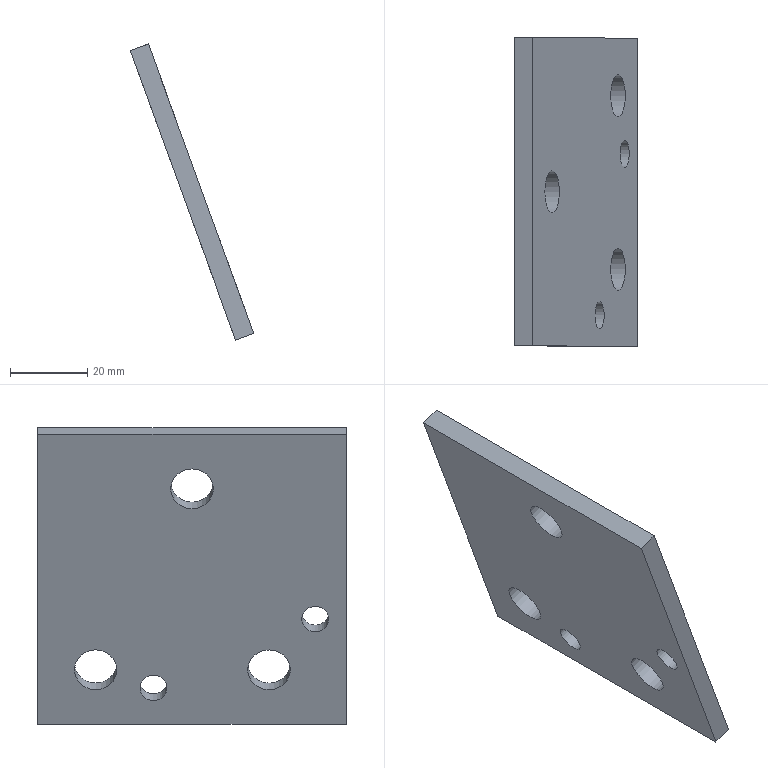Part | NX | features solid 2 | 1 solid | 11 faces | box 32.064 x 80.011 x 76.896 mm | volume 30190 mm3 | plane 6 | cylinder 5 | commonest cylinder face diameters 11 x3 7 x2
STEP:
#1=CARTESIAN_POINT('',(730.878,-346.999,86.488));
#2=VERTEX_POINT('',#1);
#3=CARTESIAN_POINT('',(758.239,-346.988,11.313));
#4=VERTEX_POINT('',#3);
#5=CARTESIAN_POINT('',(759.949,-346.987,6.614));
#6=DIRECTION('',(0.342,0.0001374,-0.9397));
#7=VECTOR('',#6,1000.);
#8=LINE('',#5,#7);
#9=EDGE_CURVE('',#2,#4,#8,.T.);
#10=ORIENTED_EDGE('',*,*,#9,.F.);
#11=CARTESIAN_POINT('',(726.179,-346.999,84.778));
#12=VERTEX_POINT('',#11);
#13=CARTESIAN_POINT('',(726.179,-346.999,84.778));
#14=DIRECTION('',(0.9397,-0.000001517,0.342));
#15=VECTOR('',#14,1000.);
#16=LINE('',#13,#15);
#17=EDGE_CURVE('',#12,#2,#16,.T.);
#18=ORIENTED_EDGE('',*,*,#17,.F.);
#19=CARTESIAN_POINT('',(753.541,-346.988,9.603));
#20=VERTEX_POINT('',#19);
#21=CARTESIAN_POINT('',(755.251,-346.987,4.904));
#22=DIRECTION('',(0.342,0.0001374,-0.9397));
#23=VECTOR('',#22,1000.);
#24=LINE('',#21,#23);
#25=EDGE_CURVE('',#12,#20,#24,.T.);
#26=ORIENTED_EDGE('',*,*,#25,.T.);
#27=CARTESIAN_POINT('',(753.541,-346.988,9.603));
#28=DIRECTION('',(0.9397,-0.000001517,0.342));
#29=VECTOR('',#28,1000.);
#30=LINE('',#27,#29);
#31=EDGE_CURVE('',#20,#4,#30,.T.);
#32=ORIENTED_EDGE('',*,*,#31,.T.);
#33=EDGE_LOOP('',(#10,#18,#26,#32));
#34=FACE_BOUND('',#33,.T.);
#35=CARTESIAN_POINT('',(755.251,-346.987,4.904));
#36=DIRECTION('',(-0.00004556,1.,0.0001296));
#37=DIRECTION('',(0.000000501,-0.0001296,1.));
#38=AXIS2_PLACEMENT_3D('',#35,#36,#37);
#39=PLANE('',#38);
#40=ADVANCED_FACE('',(#34),#39,.F.);
#41=CARTESIAN_POINT('',(730.874,-266.999,86.498));
#42=VERTEX_POINT('',#41);
#43=CARTESIAN_POINT('',(730.873,-236.999,86.502));
#44=DIRECTION('',(0.00004556,-1.,-0.0001296));
#45=VECTOR('',#44,1000.);
#46=LINE('',#43,#45);
#47=EDGE_CURVE('',#42,#2,#46,.T.);
#48=ORIENTED_EDGE('',*,*,#47,.F.);
#49=CARTESIAN_POINT('',(726.176,-266.999,84.788));
#50=VERTEX_POINT('',#49);
#51=CARTESIAN_POINT('',(726.176,-266.999,84.788));
#52=DIRECTION('',(0.9397,-0.000001517,0.342));
#53=VECTOR('',#52,1000.);
#54=LINE('',#51,#53);
#55=EDGE_CURVE('',#50,#42,#54,.T.);
#56=ORIENTED_EDGE('',*,*,#55,.F.);
#57=CARTESIAN_POINT('',(726.174,-236.999,84.792));
#58=DIRECTION('',(0.00004556,-1.,-0.0001296));
#59=VECTOR('',#58,1000.);
#60=LINE('',#57,#59);
#61=EDGE_CURVE('',#50,#12,#60,.T.);
#62=ORIENTED_EDGE('',*,*,#61,.T.);
#63=ORIENTED_EDGE('',*,*,#17,.T.);
#64=EDGE_LOOP('',(#48,#56,#62,#63));
#65=FACE_BOUND('',#64,.T.);
#66=CARTESIAN_POINT('',(726.174,-236.999,84.792));
#67=DIRECTION('',(0.342,0.0001374,-0.9397));
#68=DIRECTION('',(0.9397,-0.000001517,0.342));
#69=AXIS2_PLACEMENT_3D('',#66,#67,#68);
#70=PLANE('',#69);
#71=ADVANCED_FACE('',(#65),#70,.F.);
#72=CARTESIAN_POINT('',(758.236,-266.988,11.323));
#73=VERTEX_POINT('',#72);
#74=CARTESIAN_POINT('',(759.946,-266.987,6.625));
#75=DIRECTION('',(-0.342,-0.0001374,0.9397));
#76=VECTOR('',#75,1000.);
#77=LINE('',#74,#76);
#78=EDGE_CURVE('',#73,#42,#77,.T.);
#79=ORIENTED_EDGE('',*,*,#78,.F.);
#80=CARTESIAN_POINT('',(753.537,-266.988,9.613));
#81=VERTEX_POINT('',#80);
#82=CARTESIAN_POINT('',(753.537,-266.988,9.613));
#83=DIRECTION('',(0.9397,-0.000001517,0.342));
#84=VECTOR('',#83,1000.);
#85=LINE('',#82,#84);
#86=EDGE_CURVE('',#81,#73,#85,.T.);
#87=ORIENTED_EDGE('',*,*,#86,.F.);
#88=CARTESIAN_POINT('',(755.247,-266.987,4.914));
#89=DIRECTION('',(-0.342,-0.0001374,0.9397));
#90=VECTOR('',#89,1000.);
#91=LINE('',#88,#90);
#92=EDGE_CURVE('',#81,#50,#91,.T.);
#93=ORIENTED_EDGE('',*,*,#92,.T.);
#94=ORIENTED_EDGE('',*,*,#55,.T.);
#95=EDGE_LOOP('',(#79,#87,#93,#94));
#96=FACE_BOUND('',#95,.T.);
#97=CARTESIAN_POINT('',(755.247,-266.987,4.914));
#98=DIRECTION('',(0.00004556,-1.,-0.0001296));
#99=DIRECTION('',(-0.000000501,0.0001296,-1.));
#100=AXIS2_PLACEMENT_3D('',#97,#98,#99);
#101=PLANE('',#100);
#102=ADVANCED_FACE('',(#96),#101,.F.);
#103=CARTESIAN_POINT('',(758.234,-236.988,11.327));
#104=DIRECTION('',(-0.00004556,1.,0.0001296));
#105=VECTOR('',#104,1000.);
#106=LINE('',#103,#105);
#107=EDGE_CURVE('',#4,#73,#106,.T.);
#108=ORIENTED_EDGE('',*,*,#107,.F.);
#109=ORIENTED_EDGE('',*,*,#31,.F.);
#110=CARTESIAN_POINT('',(753.536,-236.988,9.617));
#111=DIRECTION('',(-0.00004556,1.,0.0001296));
#112=VECTOR('',#111,1000.);
#113=LINE('',#110,#112);
#114=EDGE_CURVE('',#20,#81,#113,.T.);
#115=ORIENTED_EDGE('',*,*,#114,.T.);
#116=ORIENTED_EDGE('',*,*,#86,.T.);
#117=EDGE_LOOP('',(#108,#109,#115,#116));
#118=FACE_BOUND('',#117,.T.);
#119=CARTESIAN_POINT('',(753.536,-236.988,9.617));
#120=DIRECTION('',(-0.342,-0.0001374,0.9397));
#121=DIRECTION('',(-0.9397,0.000001517,-0.342));
#122=AXIS2_PLACEMENT_3D('',#119,#120,#121);
#123=PLANE('',#122);
#124=ADVANCED_FACE('',(#118),#123,.F.);
#125=CARTESIAN_POINT('',(729.427,-306.997,75.856));
#126=VERTEX_POINT('',#125);
#127=CARTESIAN_POINT('',(731.308,-306.997,70.688));
#128=DIRECTION('',(-0.9397,0.000001517,-0.342));
#129=DIRECTION('',(-0.342,0.,0.9397));
#130=AXIS2_PLACEMENT_3D('',#127,#128,#129);
#131=CIRCLE('',#130,5.5);
#132=EDGE_CURVE('',#126,#126,#131,.T.);
#133=ORIENTED_EDGE('',*,*,#132,.F.);
#134=EDGE_LOOP('',(#133));
#135=FACE_BOUND('',#134,.T.);
#136=CARTESIAN_POINT('',(742.425,-338.992,40.144));
#137=VERTEX_POINT('',#136);
#138=CARTESIAN_POINT('',(743.622,-338.992,36.855));
#139=DIRECTION('',(-0.9397,0.000001517,-0.342));
#140=DIRECTION('',(-0.342,0.,0.9397));
#141=AXIS2_PLACEMENT_3D('',#138,#139,#140);
#142=CIRCLE('',#141,3.5);
#143=EDGE_CURVE('',#137,#137,#142,.T.);
#144=ORIENTED_EDGE('',*,*,#143,.F.);
#145=EDGE_LOOP('',(#144));
#146=FACE_BOUND('',#145,.T.);
#147=CARTESIAN_POINT('',(746.528,-326.99,28.869));
#148=VERTEX_POINT('',#147);
#149=CARTESIAN_POINT('',(748.41,-326.99,23.701));
#150=DIRECTION('',(-0.9397,0.000001517,-0.342));
#151=DIRECTION('',(-0.342,0.00000071,0.9397));
#152=AXIS2_PLACEMENT_3D('',#149,#150,#151);
#153=CIRCLE('',#152,5.5);
#154=EDGE_CURVE('',#148,#148,#153,.T.);
#155=ORIENTED_EDGE('',*,*,#154,.F.);
#156=EDGE_LOOP('',(#155));
#157=FACE_BOUND('',#156,.T.);
#158=CARTESIAN_POINT('',(748.921,-296.989,22.295));
#159=VERTEX_POINT('',#158);
#160=CARTESIAN_POINT('',(750.118,-296.989,19.006));
#161=DIRECTION('',(-0.9397,0.000001517,-0.342));
#162=DIRECTION('',(-0.342,0.,0.9397));
#163=AXIS2_PLACEMENT_3D('',#160,#161,#162);
#164=CIRCLE('',#163,3.5);
#165=EDGE_CURVE('',#159,#159,#164,.T.);
#166=ORIENTED_EDGE('',*,*,#165,.F.);
#167=EDGE_LOOP('',(#166));
#168=FACE_BOUND('',#167,.T.);
#169=CARTESIAN_POINT('',(746.526,-281.99,28.875));
#170=VERTEX_POINT('',#169);
#171=CARTESIAN_POINT('',(748.407,-281.99,23.706));
#172=DIRECTION('',(-0.9397,0.000001517,-0.342));
#173=DIRECTION('',(-0.342,0.00000071,0.9397));
#174=AXIS2_PLACEMENT_3D('',#171,#172,#173);
#175=CIRCLE('',#174,5.5);
#176=EDGE_CURVE('',#170,#170,#175,.T.);
#177=ORIENTED_EDGE('',*,*,#176,.F.);
#178=EDGE_LOOP('',(#177));
#179=FACE_BOUND('',#178,.T.);
#180=ORIENTED_EDGE('',*,*,#25,.F.);
#181=ORIENTED_EDGE('',*,*,#61,.F.);
#182=ORIENTED_EDGE('',*,*,#92,.F.);
#183=ORIENTED_EDGE('',*,*,#114,.F.);
#184=EDGE_LOOP('',(#180,#181,#182,#183));
#185=FACE_BOUND('',#184,.T.);
#186=CARTESIAN_POINT('',(755.246,-236.987,4.918));
#187=DIRECTION('',(0.9397,-0.000001517,0.342));
#188=DIRECTION('',(-0.342,-0.0001374,0.9397));
#189=AXIS2_PLACEMENT_3D('',#186,#187,#188);
#190=PLANE('',#189);
#191=ADVANCED_FACE('',(#135,#146,#157,#168,#179,#185),#190,.F.);
#192=CARTESIAN_POINT('',(734.125,-306.997,77.566));
#193=VERTEX_POINT('',#192);
#194=CARTESIAN_POINT('',(736.006,-306.997,72.398));
#195=DIRECTION('',(-0.9397,0.000001517,-0.342));
#196=DIRECTION('',(-0.342,0.,0.9397));
#197=AXIS2_PLACEMENT_3D('',#194,#195,#196);
#198=CIRCLE('',#197,5.5);
#199=EDGE_CURVE('',#193,#193,#198,.T.);
#200=ORIENTED_EDGE('',*,*,#199,.T.);
#201=EDGE_LOOP('',(#200));
#202=FACE_BOUND('',#201,.T.);
#203=CARTESIAN_POINT('',(747.123,-338.992,41.854));
#204=VERTEX_POINT('',#203);
#205=CARTESIAN_POINT('',(748.32,-338.992,38.565));
#206=DIRECTION('',(-0.9397,0.000001517,-0.342));
#207=DIRECTION('',(-0.342,0.,0.9397));
#208=AXIS2_PLACEMENT_3D('',#205,#206,#207);
#209=CIRCLE('',#208,3.5);
#210=EDGE_CURVE('',#204,#204,#209,.T.);
#211=ORIENTED_EDGE('',*,*,#210,.T.);
#212=EDGE_LOOP('',(#211));
#213=FACE_BOUND('',#212,.T.);
#214=CARTESIAN_POINT('',(751.227,-326.99,30.579));
#215=VERTEX_POINT('',#214);
#216=CARTESIAN_POINT('',(753.108,-326.99,25.411));
#217=DIRECTION('',(-0.9397,0.000001517,-0.342));
#218=DIRECTION('',(-0.342,0.00000071,0.9397));
#219=AXIS2_PLACEMENT_3D('',#216,#217,#218);
#220=CIRCLE('',#219,5.5);
#221=EDGE_CURVE('',#215,#215,#220,.T.);
#222=ORIENTED_EDGE('',*,*,#221,.T.);
#223=EDGE_LOOP('',(#222));
#224=FACE_BOUND('',#223,.T.);
#225=CARTESIAN_POINT('',(753.62,-296.989,24.005));
#226=VERTEX_POINT('',#225);
#227=CARTESIAN_POINT('',(754.817,-296.989,20.716));
#228=DIRECTION('',(-0.9397,0.000001517,-0.342));
#229=DIRECTION('',(-0.342,0.,0.9397));
#230=AXIS2_PLACEMENT_3D('',#227,#228,#229);
#231=CIRCLE('',#230,3.5);
#232=EDGE_CURVE('',#226,#226,#231,.T.);
#233=ORIENTED_EDGE('',*,*,#232,.T.);
#234=EDGE_LOOP('',(#233));
#235=FACE_BOUND('',#234,.T.);
#236=CARTESIAN_POINT('',(751.225,-281.99,30.585));
#237=VERTEX_POINT('',#236);
#238=CARTESIAN_POINT('',(753.106,-281.99,25.416));
#239=DIRECTION('',(-0.9397,0.000001517,-0.342));
#240=DIRECTION('',(-0.342,0.00000071,0.9397));
#241=AXIS2_PLACEMENT_3D('',#238,#239,#240);
#242=CIRCLE('',#241,5.5);
#243=EDGE_CURVE('',#237,#237,#242,.T.);
#244=ORIENTED_EDGE('',*,*,#243,.T.);
#245=EDGE_LOOP('',(#244));
#246=FACE_BOUND('',#245,.T.);
#247=ORIENTED_EDGE('',*,*,#9,.T.);
#248=ORIENTED_EDGE('',*,*,#107,.T.);
#249=ORIENTED_EDGE('',*,*,#78,.T.);
#250=ORIENTED_EDGE('',*,*,#47,.T.);
#251=EDGE_LOOP('',(#247,#248,#249,#250));
#252=FACE_BOUND('',#251,.T.);
#253=CARTESIAN_POINT('',(759.944,-236.987,6.628));
#254=DIRECTION('',(0.9397,-0.000001517,0.342));
#255=DIRECTION('',(-0.342,-0.0001374,0.9397));
#256=AXIS2_PLACEMENT_3D('',#253,#254,#255);
#257=PLANE('',#256);
#258=ADVANCED_FACE('',(#202,#213,#224,#235,#246,#252),#257,.T.);
#259=ORIENTED_EDGE('',*,*,#243,.F.);
#260=EDGE_LOOP('',(#259));
#261=FACE_BOUND('',#260,.T.);
#262=ORIENTED_EDGE('',*,*,#176,.T.);
#263=EDGE_LOOP('',(#262));
#264=FACE_BOUND('',#263,.T.);
#265=CARTESIAN_POINT('',(743.709,-281.99,21.996));
#266=DIRECTION('',(0.9397,-0.000001517,0.342));
#267=DIRECTION('',(-0.342,0.00000071,0.9397));
#268=AXIS2_PLACEMENT_3D('',#265,#266,#267);
#269=CYLINDRICAL_SURFACE('',#268,5.5);
#270=ADVANCED_FACE('',(#261,#264),#269,.F.);
#271=ORIENTED_EDGE('',*,*,#232,.F.);
#272=EDGE_LOOP('',(#271));
#273=FACE_BOUND('',#272,.T.);
#274=ORIENTED_EDGE('',*,*,#165,.T.);
#275=EDGE_LOOP('',(#274));
#276=FACE_BOUND('',#275,.T.);
#277=CARTESIAN_POINT('',(745.42,-296.989,17.296));
#278=DIRECTION('',(0.9397,-0.000001517,0.342));
#279=DIRECTION('',(-0.342,0.00000071,0.9397));
#280=AXIS2_PLACEMENT_3D('',#277,#278,#279);
#281=CYLINDRICAL_SURFACE('',#280,3.5);
#282=ADVANCED_FACE('',(#273,#276),#281,.F.);
#283=ORIENTED_EDGE('',*,*,#221,.F.);
#284=EDGE_LOOP('',(#283));
#285=FACE_BOUND('',#284,.T.);
#286=ORIENTED_EDGE('',*,*,#154,.T.);
#287=EDGE_LOOP('',(#286));
#288=FACE_BOUND('',#287,.T.);
#289=CARTESIAN_POINT('',(743.711,-326.99,21.99));
#290=DIRECTION('',(0.9397,-0.000001517,0.342));
#291=DIRECTION('',(-0.342,0.00000071,0.9397));
#292=AXIS2_PLACEMENT_3D('',#289,#290,#291);
#293=CYLINDRICAL_SURFACE('',#292,5.5);
#294=ADVANCED_FACE('',(#285,#288),#293,.F.);
#295=ORIENTED_EDGE('',*,*,#210,.F.);
#296=EDGE_LOOP('',(#295));
#297=FACE_BOUND('',#296,.T.);
#298=ORIENTED_EDGE('',*,*,#143,.T.);
#299=EDGE_LOOP('',(#298));
#300=FACE_BOUND('',#299,.T.);
#301=CARTESIAN_POINT('',(738.923,-338.992,35.145));
#302=DIRECTION('',(0.9397,-0.000001517,0.342));
#303=DIRECTION('',(-0.342,0.00000071,0.9397));
#304=AXIS2_PLACEMENT_3D('',#301,#302,#303);
#305=CYLINDRICAL_SURFACE('',#304,3.5);
#306=ADVANCED_FACE('',(#297,#300),#305,.F.);
#307=ORIENTED_EDGE('',*,*,#199,.F.);
#308=EDGE_LOOP('',(#307));
#309=FACE_BOUND('',#308,.T.);
#310=ORIENTED_EDGE('',*,*,#132,.T.);
#311=EDGE_LOOP('',(#310));
#312=FACE_BOUND('',#311,.T.);
#313=CARTESIAN_POINT('',(620.424,-306.997,30.329));
#314=DIRECTION('',(0.9397,-0.000001517,0.342));
#315=DIRECTION('',(-0.342,0.,0.9397));
#316=AXIS2_PLACEMENT_3D('',#313,#314,#315);
#317=CYLINDRICAL_SURFACE('',#316,5.5);
#318=ADVANCED_FACE('',(#309,#312),#317,.F.);
#319=CLOSED_SHELL('',(#40,#71,#102,#124,#191,#258,#270,#282,#294,#306,#318));
#320=MANIFOLD_SOLID_BREP('',#319);
#321=(LENGTH_UNIT()NAMED_UNIT(*)SI_UNIT(.MILLI.,.METRE.));
#322=UNCERTAINTY_MEASURE_WITH_UNIT(LENGTH_MEASURE(0.00001),#321,'','');
#323=(NAMED_UNIT(*)PLANE_ANGLE_UNIT()SI_UNIT($,.RADIAN.));
#324=(NAMED_UNIT(*)SI_UNIT($,.STERADIAN.)SOLID_ANGLE_UNIT());
#325=(GEOMETRIC_REPRESENTATION_CONTEXT(3)GLOBAL_UNCERTAINTY_ASSIGNED_CONTEXT((#322))GLOBAL_UNIT_ASSIGNED_CONTEXT((#321,#323,#324))REPRESENTATION_CONTEXT('',''));
#326=ADVANCED_BREP_SHAPE_REPRESENTATION('',(#320),#325);